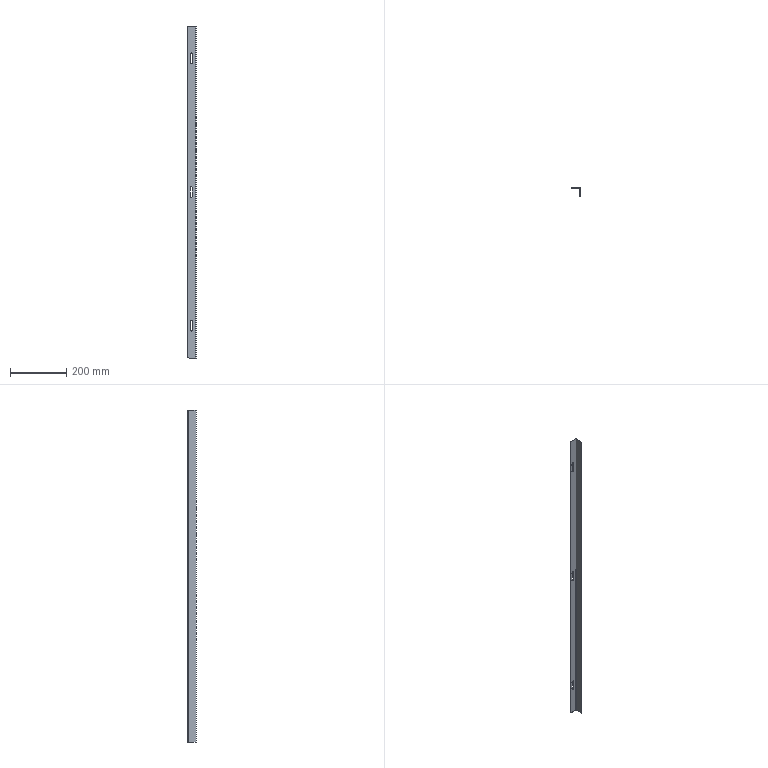Part | SolidWorks | features Cut 1, Fillet 1, FlatPattern 1, SMBaseFlange 1, SheetMetal 1 | 1 solid | 31 faces | box 30 x 30 x 1181 mm | volume 101588 mm3 | plane 18 | cylinder 13 | commonest cylinder face diameters 8 x9 10 x2 0.4 x1 3.4 x1
STEP:
#1=CARTESIAN_POINT('',(-17.5,-1.5,494.5));
#2=VERTEX_POINT('',#1);
#3=CARTESIAN_POINT('',(-13.5,-1.5,490.5));
#4=VERTEX_POINT('',#3);
#5=CARTESIAN_POINT('',(-17.5,-1.5,490.5));
#6=DIRECTION('',(0.,1.,0.));
#7=DIRECTION('',(-1.,0.,0.));
#8=AXIS2_PLACEMENT_3D('',#5,#6,#7);
#9=CIRCLE('',#8,4.);
#10=EDGE_CURVE('',#2,#4,#9,.T.);
#11=ORIENTED_EDGE('',*,*,#10,.F.);
#12=CARTESIAN_POINT('',(-17.5,0.,494.5));
#13=VERTEX_POINT('',#12);
#14=CARTESIAN_POINT('',(-17.5,-10.,494.5));
#15=DIRECTION('',(0.,1.,0.));
#16=VECTOR('',#15,1000.);
#17=LINE('',#14,#16);
#18=EDGE_CURVE('',#2,#13,#17,.T.);
#19=ORIENTED_EDGE('',*,*,#18,.T.);
#20=CARTESIAN_POINT('',(-13.5,0.,490.5));
#21=VERTEX_POINT('',#20);
#22=CARTESIAN_POINT('',(-17.5,0.,490.5));
#23=DIRECTION('',(0.,1.,0.));
#24=DIRECTION('',(0.,0.,-1.));
#25=AXIS2_PLACEMENT_3D('',#22,#23,#24);
#26=CIRCLE('',#25,4.);
#27=EDGE_CURVE('',#13,#21,#26,.T.);
#28=ORIENTED_EDGE('',*,*,#27,.T.);
#29=CARTESIAN_POINT('',(-13.5,-10.,490.5));
#30=DIRECTION('',(0.,1.,0.));
#31=VECTOR('',#30,1000.);
#32=LINE('',#29,#31);
#33=EDGE_CURVE('',#4,#21,#32,.T.);
#34=ORIENTED_EDGE('',*,*,#33,.F.);
#35=EDGE_LOOP('',(#11,#19,#28,#34));
#36=FACE_OUTER_BOUND('',#35,.T.);
#37=CARTESIAN_POINT('',(-17.5,-10.,490.5));
#38=DIRECTION('',(0.,1.,0.));
#39=DIRECTION('',(0.,0.,1.));
#40=AXIS2_PLACEMENT_3D('',#37,#38,#39);
#41=CYLINDRICAL_SURFACE('',#40,4.);
#42=ADVANCED_FACE('',(#36),#41,.F.);
#43=CARTESIAN_POINT('',(-17.5,-1.5,-456.5));
#44=VERTEX_POINT('',#43);
#45=CARTESIAN_POINT('',(-13.5,-1.5,-460.5));
#46=VERTEX_POINT('',#45);
#47=CARTESIAN_POINT('',(-17.5,-1.5,-460.5));
#48=DIRECTION('',(0.,1.,0.));
#49=DIRECTION('',(-1.,0.,0.));
#50=AXIS2_PLACEMENT_3D('',#47,#48,#49);
#51=CIRCLE('',#50,4.);
#52=EDGE_CURVE('',#44,#46,#51,.T.);
#53=ORIENTED_EDGE('',*,*,#52,.F.);
#54=CARTESIAN_POINT('',(-17.5,0.,-456.5));
#55=VERTEX_POINT('',#54);
#56=CARTESIAN_POINT('',(-17.5,-10.,-456.5));
#57=DIRECTION('',(0.,1.,0.));
#58=VECTOR('',#57,1000.);
#59=LINE('',#56,#58);
#60=EDGE_CURVE('',#44,#55,#59,.T.);
#61=ORIENTED_EDGE('',*,*,#60,.T.);
#62=CARTESIAN_POINT('',(-13.5,0.,-460.5));
#63=VERTEX_POINT('',#62);
#64=CARTESIAN_POINT('',(-17.5,0.,-460.5));
#65=DIRECTION('',(0.,1.,0.));
#66=DIRECTION('',(0.,0.,1.));
#67=AXIS2_PLACEMENT_3D('',#64,#65,#66);
#68=CIRCLE('',#67,4.);
#69=EDGE_CURVE('',#55,#63,#68,.T.);
#70=ORIENTED_EDGE('',*,*,#69,.T.);
#71=CARTESIAN_POINT('',(-13.5,-10.,-460.5));
#72=DIRECTION('',(0.,1.,0.));
#73=VECTOR('',#72,1000.);
#74=LINE('',#71,#73);
#75=EDGE_CURVE('',#46,#63,#74,.T.);
#76=ORIENTED_EDGE('',*,*,#75,.F.);
#77=EDGE_LOOP('',(#53,#61,#70,#76));
#78=FACE_OUTER_BOUND('',#77,.T.);
#79=CARTESIAN_POINT('',(-17.5,-10.,-460.5));
#80=DIRECTION('',(0.,1.,0.));
#81=DIRECTION('',(0.,0.,1.));
#82=AXIS2_PLACEMENT_3D('',#79,#80,#81);
#83=CYLINDRICAL_SURFACE('',#82,4.);
#84=ADVANCED_FACE('',(#78),#83,.F.);
#85=CARTESIAN_POINT('',(-17.5,-1.5,19.));
#86=VERTEX_POINT('',#85);
#87=CARTESIAN_POINT('',(-13.5,-1.5,15.));
#88=VERTEX_POINT('',#87);
#89=CARTESIAN_POINT('',(-17.5,-1.5,15.));
#90=DIRECTION('',(0.,1.,0.));
#91=DIRECTION('',(-1.,0.,0.));
#92=AXIS2_PLACEMENT_3D('',#89,#90,#91);
#93=CIRCLE('',#92,4.);
#94=EDGE_CURVE('',#86,#88,#93,.T.);
#95=ORIENTED_EDGE('',*,*,#94,.F.);
#96=CARTESIAN_POINT('',(-17.5,0.,19.));
#97=VERTEX_POINT('',#96);
#98=CARTESIAN_POINT('',(-17.5,-10.,19.));
#99=DIRECTION('',(0.,1.,0.));
#100=VECTOR('',#99,1000.);
#101=LINE('',#98,#100);
#102=EDGE_CURVE('',#86,#97,#101,.T.);
#103=ORIENTED_EDGE('',*,*,#102,.T.);
#104=CARTESIAN_POINT('',(-13.5,0.,15.));
#105=VERTEX_POINT('',#104);
#106=CARTESIAN_POINT('',(-17.5,0.,15.));
#107=DIRECTION('',(0.,1.,0.));
#108=DIRECTION('',(0.,0.,1.));
#109=AXIS2_PLACEMENT_3D('',#106,#107,#108);
#110=CIRCLE('',#109,4.);
#111=EDGE_CURVE('',#97,#105,#110,.T.);
#112=ORIENTED_EDGE('',*,*,#111,.T.);
#113=CARTESIAN_POINT('',(-13.5,-10.,15.));
#114=DIRECTION('',(0.,1.,0.));
#115=VECTOR('',#114,1000.);
#116=LINE('',#113,#115);
#117=EDGE_CURVE('',#88,#105,#116,.T.);
#118=ORIENTED_EDGE('',*,*,#117,.F.);
#119=EDGE_LOOP('',(#95,#103,#112,#118));
#120=FACE_OUTER_BOUND('',#119,.T.);
#121=CARTESIAN_POINT('',(-17.5,-10.,15.));
#122=DIRECTION('',(0.,1.,0.));
#123=DIRECTION('',(0.,0.,1.));
#124=AXIS2_PLACEMENT_3D('',#121,#122,#123);
#125=CYLINDRICAL_SURFACE('',#124,4.);
#126=ADVANCED_FACE('',(#120),#125,.F.);
#127=CARTESIAN_POINT('',(0.,-1.7,590.5));
#128=VERTEX_POINT('',#127);
#129=CARTESIAN_POINT('',(-1.5,-1.7,590.5));
#130=VERTEX_POINT('',#129);
#131=CARTESIAN_POINT('',(0.,-1.7,590.5));
#132=DIRECTION('',(-1.,0.,0.));
#133=VECTOR('',#132,1000.);
#134=LINE('',#131,#133);
#135=EDGE_CURVE('',#128,#130,#134,.T.);
#136=ORIENTED_EDGE('',*,*,#135,.F.);
#137=CARTESIAN_POINT('',(-1.7,0.,590.5));
#138=VERTEX_POINT('',#137);
#139=CARTESIAN_POINT('',(-1.7,-1.7,590.5));
#140=DIRECTION('',(0.,0.,-1.));
#141=DIRECTION('',(1.,0.,0.));
#142=AXIS2_PLACEMENT_3D('',#139,#140,#141);
#143=CIRCLE('',#142,1.7);
#144=EDGE_CURVE('',#138,#128,#143,.T.);
#145=ORIENTED_EDGE('',*,*,#144,.F.);
#146=CARTESIAN_POINT('',(-1.7,-1.5,590.5));
#147=VERTEX_POINT('',#146);
#148=CARTESIAN_POINT('',(-1.7,-1.5,590.5));
#149=DIRECTION('',(0.,1.,0.));
#150=VECTOR('',#149,1000.);
#151=LINE('',#148,#150);
#152=EDGE_CURVE('',#147,#138,#151,.T.);
#153=ORIENTED_EDGE('',*,*,#152,.F.);
#154=CARTESIAN_POINT('',(-1.7,-1.7,590.5));
#155=DIRECTION('',(0.,0.,-1.));
#156=DIRECTION('',(1.,0.,0.));
#157=AXIS2_PLACEMENT_3D('',#154,#155,#156);
#158=CIRCLE('',#157,0.2);
#159=EDGE_CURVE('',#147,#130,#158,.T.);
#160=ORIENTED_EDGE('',*,*,#159,.T.);
#161=EDGE_LOOP('',(#136,#145,#153,#160));
#162=FACE_OUTER_BOUND('',#161,.T.);
#163=CARTESIAN_POINT('',(0.,-1.7,590.5));
#164=DIRECTION('',(0.,0.,1.));
#165=DIRECTION('',(1.,0.,0.));
#166=AXIS2_PLACEMENT_3D('',#163,#164,#165);
#167=PLANE('',#166);
#168=ADVANCED_FACE('',(#162),#167,.T.);
#169=CARTESIAN_POINT('',(0.,-30.,590.5));
#170=VERTEX_POINT('',#169);
#171=CARTESIAN_POINT('',(0.,0.,590.5));
#172=DIRECTION('',(0.,-1.,0.));
#173=VECTOR('',#172,1000.);
#174=LINE('',#171,#173);
#175=EDGE_CURVE('',#128,#170,#174,.T.);
#176=ORIENTED_EDGE('',*,*,#175,.F.);
#177=ORIENTED_EDGE('',*,*,#135,.T.);
#178=CARTESIAN_POINT('',(-1.5,-30.,590.5));
#179=VERTEX_POINT('',#178);
#180=CARTESIAN_POINT('',(-1.5,0.,590.5));
#181=DIRECTION('',(0.,-1.,0.));
#182=VECTOR('',#181,1000.);
#183=LINE('',#180,#182);
#184=EDGE_CURVE('',#130,#179,#183,.T.);
#185=ORIENTED_EDGE('',*,*,#184,.T.);
#186=CARTESIAN_POINT('',(0.,-30.,590.5));
#187=DIRECTION('',(-1.,0.,0.));
#188=VECTOR('',#187,1000.);
#189=LINE('',#186,#188);
#190=EDGE_CURVE('',#170,#179,#189,.T.);
#191=ORIENTED_EDGE('',*,*,#190,.F.);
#192=EDGE_LOOP('',(#176,#177,#185,#191));
#193=FACE_OUTER_BOUND('',#192,.T.);
#194=CARTESIAN_POINT('',(-1.7,-1.5,590.5));
#195=DIRECTION('',(0.,0.,1.));
#196=DIRECTION('',(1.,0.,0.));
#197=AXIS2_PLACEMENT_3D('',#194,#195,#196);
#198=PLANE('',#197);
#199=ADVANCED_FACE('',(#193),#198,.T.);
#200=CARTESIAN_POINT('',(-1.7,0.,-590.5));
#201=VERTEX_POINT('',#200);
#202=CARTESIAN_POINT('',(-1.7,-1.5,-590.5));
#203=VERTEX_POINT('',#202);
#204=CARTESIAN_POINT('',(-1.7,0.,-590.5));
#205=DIRECTION('',(0.,-1.,0.));
#206=VECTOR('',#205,1000.);
#207=LINE('',#204,#206);
#208=EDGE_CURVE('',#201,#203,#207,.T.);
#209=ORIENTED_EDGE('',*,*,#208,.F.);
#210=CARTESIAN_POINT('',(0.,-1.7,-590.5));
#211=VERTEX_POINT('',#210);
#212=CARTESIAN_POINT('',(-1.7,-1.7,-590.5));
#213=DIRECTION('',(0.,0.,-1.));
#214=DIRECTION('',(1.,0.,0.));
#215=AXIS2_PLACEMENT_3D('',#212,#213,#214);
#216=CIRCLE('',#215,1.7);
#217=EDGE_CURVE('',#201,#211,#216,.T.);
#218=ORIENTED_EDGE('',*,*,#217,.T.);
#219=CARTESIAN_POINT('',(-1.5,-1.7,-590.5));
#220=VERTEX_POINT('',#219);
#221=CARTESIAN_POINT('',(-1.5,-1.7,-590.5));
#222=DIRECTION('',(1.,0.,0.));
#223=VECTOR('',#222,1000.);
#224=LINE('',#221,#223);
#225=EDGE_CURVE('',#220,#211,#224,.T.);
#226=ORIENTED_EDGE('',*,*,#225,.F.);
#227=CARTESIAN_POINT('',(-1.7,-1.7,-590.5));
#228=DIRECTION('',(0.,0.,-1.));
#229=DIRECTION('',(1.,0.,0.));
#230=AXIS2_PLACEMENT_3D('',#227,#228,#229);
#231=CIRCLE('',#230,0.2);
#232=EDGE_CURVE('',#203,#220,#231,.T.);
#233=ORIENTED_EDGE('',*,*,#232,.F.);
#234=EDGE_LOOP('',(#209,#218,#226,#233));
#235=FACE_OUTER_BOUND('',#234,.T.);
#236=CARTESIAN_POINT('',(-1.7,0.,-590.5));
#237=DIRECTION('',(0.,0.,-1.));
#238=DIRECTION('',(-1.,0.,0.));
#239=AXIS2_PLACEMENT_3D('',#236,#237,#238);
#240=PLANE('',#239);
#241=ADVANCED_FACE('',(#235),#240,.T.);
#242=CARTESIAN_POINT('',(-25.,-1.5,-590.5));
#243=VERTEX_POINT('',#242);
#244=CARTESIAN_POINT('',(0.,-1.5,-590.5));
#245=DIRECTION('',(1.,0.,0.));
#246=VECTOR('',#245,1000.);
#247=LINE('',#244,#246);
#248=EDGE_CURVE('',#243,#203,#247,.T.);
#249=ORIENTED_EDGE('',*,*,#248,.F.);
#250=CARTESIAN_POINT('',(-25.,0.,-590.5));
#251=VERTEX_POINT('',#250);
#252=CARTESIAN_POINT('',(-25.,-1.7,-590.5));
#253=DIRECTION('',(0.,1.,0.));
#254=VECTOR('',#253,1000.);
#255=LINE('',#252,#254);
#256=EDGE_CURVE('',#243,#251,#255,.T.);
#257=ORIENTED_EDGE('',*,*,#256,.T.);
#258=CARTESIAN_POINT('',(0.,0.,-590.5));
#259=DIRECTION('',(1.,0.,0.));
#260=VECTOR('',#259,1000.);
#261=LINE('',#258,#260);
#262=EDGE_CURVE('',#251,#201,#261,.T.);
#263=ORIENTED_EDGE('',*,*,#262,.T.);
#264=ORIENTED_EDGE('',*,*,#208,.T.);
#265=EDGE_LOOP('',(#249,#257,#263,#264));
#266=FACE_OUTER_BOUND('',#265,.T.);
#267=CARTESIAN_POINT('',(-1.5,-1.7,-590.5));
#268=DIRECTION('',(0.,0.,-1.));
#269=DIRECTION('',(-1.,0.,0.));
#270=AXIS2_PLACEMENT_3D('',#267,#268,#269);
#271=PLANE('',#270);
#272=ADVANCED_FACE('',(#266),#271,.T.);
#273=CARTESIAN_POINT('',(-1.5,-30.,-590.5));
#274=VERTEX_POINT('',#273);
#275=CARTESIAN_POINT('',(-1.5,0.,-590.5));
#276=DIRECTION('',(0.,-1.,0.));
#277=VECTOR('',#276,1000.);
#278=LINE('',#275,#277);
#279=EDGE_CURVE('',#220,#274,#278,.T.);
#280=ORIENTED_EDGE('',*,*,#279,.T.);
#281=CARTESIAN_POINT('',(-1.5,-30.,590.5));
#282=DIRECTION('',(0.,0.,-1.));
#283=VECTOR('',#282,1000.);
#284=LINE('',#281,#283);
#285=EDGE_CURVE('',#179,#274,#284,.T.);
#286=ORIENTED_EDGE('',*,*,#285,.F.);
#287=ORIENTED_EDGE('',*,*,#184,.F.);
#288=CARTESIAN_POINT('',(-1.5,-1.7,590.5));
#289=DIRECTION('',(0.,0.,-1.));
#290=VECTOR('',#289,1000.);
#291=LINE('',#288,#290);
#292=EDGE_CURVE('',#130,#220,#291,.T.);
#293=ORIENTED_EDGE('',*,*,#292,.T.);
#294=EDGE_LOOP('',(#280,#286,#287,#293));
#295=FACE_OUTER_BOUND('',#294,.T.);
#296=CARTESIAN_POINT('',(-1.5,0.,590.5));
#297=DIRECTION('',(1.,0.,0.));
#298=DIRECTION('',(0.,1.,0.));
#299=AXIS2_PLACEMENT_3D('',#296,#297,#298);
#300=PLANE('',#299);
#301=ADVANCED_FACE('',(#295),#300,.F.);
#302=CARTESIAN_POINT('',(0.,-30.,-590.5));
#303=VERTEX_POINT('',#302);
#304=CARTESIAN_POINT('',(0.,-30.,-590.5));
#305=DIRECTION('',(-1.,0.,0.));
#306=VECTOR('',#305,1000.);
#307=LINE('',#304,#306);
#308=EDGE_CURVE('',#303,#274,#307,.T.);
#309=ORIENTED_EDGE('',*,*,#308,.F.);
#310=CARTESIAN_POINT('',(0.,-30.,590.5));
#311=DIRECTION('',(0.,0.,-1.));
#312=VECTOR('',#311,1000.);
#313=LINE('',#310,#312);
#314=EDGE_CURVE('',#170,#303,#313,.T.);
#315=ORIENTED_EDGE('',*,*,#314,.F.);
#316=ORIENTED_EDGE('',*,*,#190,.T.);
#317=ORIENTED_EDGE('',*,*,#285,.T.);
#318=EDGE_LOOP('',(#309,#315,#316,#317));
#319=FACE_OUTER_BOUND('',#318,.T.);
#320=CARTESIAN_POINT('',(0.,-30.,590.5));
#321=DIRECTION('',(0.,-1.,0.));
#322=DIRECTION('',(0.,0.,-1.));
#323=AXIS2_PLACEMENT_3D('',#320,#321,#322);
#324=PLANE('',#323);
#325=ADVANCED_FACE('',(#319),#324,.T.);
#326=CARTESIAN_POINT('',(0.,0.,-590.5));
#327=DIRECTION('',(0.,-1.,0.));
#328=VECTOR('',#327,1000.);
#329=LINE('',#326,#328);
#330=EDGE_CURVE('',#211,#303,#329,.T.);
#331=ORIENTED_EDGE('',*,*,#330,.F.);
#332=CARTESIAN_POINT('',(0.,-1.7,590.5));
#333=DIRECTION('',(0.,0.,-1.));
#334=VECTOR('',#333,1000.);
#335=LINE('',#332,#334);
#336=EDGE_CURVE('',#128,#211,#335,.T.);
#337=ORIENTED_EDGE('',*,*,#336,.F.);
#338=ORIENTED_EDGE('',*,*,#175,.T.);
#339=ORIENTED_EDGE('',*,*,#314,.T.);
#340=EDGE_LOOP('',(#331,#337,#338,#339));
#341=FACE_OUTER_BOUND('',#340,.T.);
#342=CARTESIAN_POINT('',(0.,0.,590.5));
#343=DIRECTION('',(1.,0.,0.));
#344=DIRECTION('',(0.,1.,0.));
#345=AXIS2_PLACEMENT_3D('',#342,#343,#344);
#346=PLANE('',#345);
#347=ADVANCED_FACE('',(#341),#346,.T.);
#348=ORIENTED_EDGE('',*,*,#217,.F.);
#349=CARTESIAN_POINT('',(-1.7,0.,590.5));
#350=DIRECTION('',(0.,0.,-1.));
#351=VECTOR('',#350,1000.);
#352=LINE('',#349,#351);
#353=EDGE_CURVE('',#138,#201,#352,.T.);
#354=ORIENTED_EDGE('',*,*,#353,.F.);
#355=ORIENTED_EDGE('',*,*,#144,.T.);
#356=ORIENTED_EDGE('',*,*,#336,.T.);
#357=EDGE_LOOP('',(#348,#354,#355,#356));
#358=FACE_OUTER_BOUND('',#357,.T.);
#359=CARTESIAN_POINT('',(-1.7,-1.7,590.5));
#360=DIRECTION('',(0.,0.,-1.));
#361=DIRECTION('',(-1.,0.,0.));
#362=AXIS2_PLACEMENT_3D('',#359,#360,#361);
#363=CYLINDRICAL_SURFACE('',#362,1.7);
#364=ADVANCED_FACE('',(#358),#363,.T.);
#365=CARTESIAN_POINT('',(-13.5,0.,460.5));
#366=VERTEX_POINT('',#365);
#367=CARTESIAN_POINT('',(-21.5,0.,460.5));
#368=VERTEX_POINT('',#367);
#369=CARTESIAN_POINT('',(-17.5,0.,460.5));
#370=DIRECTION('',(0.,1.,0.));
#371=DIRECTION('',(0.,0.,-1.));
#372=AXIS2_PLACEMENT_3D('',#369,#370,#371);
#373=CIRCLE('',#372,4.);
#374=EDGE_CURVE('',#366,#368,#373,.T.);
#375=ORIENTED_EDGE('',*,*,#374,.F.);
#376=CARTESIAN_POINT('',(-13.5,0.,460.5));
#377=DIRECTION('',(0.,0.,-1.));
#378=VECTOR('',#377,1000.);
#379=LINE('',#376,#378);
#380=EDGE_CURVE('',#21,#366,#379,.T.);
#381=ORIENTED_EDGE('',*,*,#380,.F.);
#382=ORIENTED_EDGE('',*,*,#27,.F.);
#383=CARTESIAN_POINT('',(-21.5,0.,490.5));
#384=VERTEX_POINT('',#383);
#385=CARTESIAN_POINT('',(-17.5,0.,490.5));
#386=DIRECTION('',(0.,1.,0.));
#387=DIRECTION('',(0.,0.,-1.));
#388=AXIS2_PLACEMENT_3D('',#385,#386,#387);
#389=CIRCLE('',#388,4.);
#390=EDGE_CURVE('',#384,#13,#389,.T.);
#391=ORIENTED_EDGE('',*,*,#390,.F.);
#392=CARTESIAN_POINT('',(-21.5,0.,460.5));
#393=DIRECTION('',(0.,0.,1.));
#394=VECTOR('',#393,1000.);
#395=LINE('',#392,#394);
#396=EDGE_CURVE('',#368,#384,#395,.T.);
#397=ORIENTED_EDGE('',*,*,#396,.F.);
#398=EDGE_LOOP('',(#375,#381,#382,#391,#397));
#399=FACE_BOUND('',#398,.T.);
#400=CARTESIAN_POINT('',(-21.5,0.,-460.5));
#401=VERTEX_POINT('',#400);
#402=CARTESIAN_POINT('',(-17.5,0.,-460.5));
#403=DIRECTION('',(0.,1.,0.));
#404=DIRECTION('',(0.,0.,1.));
#405=AXIS2_PLACEMENT_3D('',#402,#403,#404);
#406=CIRCLE('',#405,4.);
#407=EDGE_CURVE('',#401,#55,#406,.T.);
#408=ORIENTED_EDGE('',*,*,#407,.F.);
#409=CARTESIAN_POINT('',(-21.5,0.,-490.5));
#410=VERTEX_POINT('',#409);
#411=CARTESIAN_POINT('',(-21.5,0.,-460.5));
#412=DIRECTION('',(0.,0.,1.));
#413=VECTOR('',#412,1000.);
#414=LINE('',#411,#413);
#415=EDGE_CURVE('',#410,#401,#414,.T.);
#416=ORIENTED_EDGE('',*,*,#415,.F.);
#417=CARTESIAN_POINT('',(-13.5,0.,-490.5));
#418=VERTEX_POINT('',#417);
#419=CARTESIAN_POINT('',(-17.5,0.,-490.5));
#420=DIRECTION('',(0.,1.,0.));
#421=DIRECTION('',(0.,0.,1.));
#422=AXIS2_PLACEMENT_3D('',#419,#420,#421);
#423=CIRCLE('',#422,4.);
#424=EDGE_CURVE('',#418,#410,#423,.T.);
#425=ORIENTED_EDGE('',*,*,#424,.F.);
#426=CARTESIAN_POINT('',(-13.5,0.,-460.5));
#427=DIRECTION('',(0.,0.,-1.));
#428=VECTOR('',#427,1000.);
#429=LINE('',#426,#428);
#430=EDGE_CURVE('',#63,#418,#429,.T.);
#431=ORIENTED_EDGE('',*,*,#430,.F.);
#432=ORIENTED_EDGE('',*,*,#69,.F.);
#433=EDGE_LOOP('',(#408,#416,#425,#431,#432));
#434=FACE_BOUND('',#433,.T.);
#435=CARTESIAN_POINT('',(-21.5,0.,15.));
#436=VERTEX_POINT('',#435);
#437=CARTESIAN_POINT('',(-17.5,0.,15.));
#438=DIRECTION('',(0.,1.,0.));
#439=DIRECTION('',(0.,0.,1.));
#440=AXIS2_PLACEMENT_3D('',#437,#438,#439);
#441=CIRCLE('',#440,4.);
#442=EDGE_CURVE('',#436,#97,#441,.T.);
#443=ORIENTED_EDGE('',*,*,#442,.F.);
#444=CARTESIAN_POINT('',(-21.5,0.,-15.));
#445=VERTEX_POINT('',#444);
#446=CARTESIAN_POINT('',(-21.5,0.,15.));
#447=DIRECTION('',(0.,0.,1.));
#448=VECTOR('',#447,1000.);
#449=LINE('',#446,#448);
#450=EDGE_CURVE('',#445,#436,#449,.T.);
#451=ORIENTED_EDGE('',*,*,#450,.F.);
#452=CARTESIAN_POINT('',(-13.5,0.,-15.));
#453=VERTEX_POINT('',#452);
#454=CARTESIAN_POINT('',(-17.5,0.,-15.));
#455=DIRECTION('',(0.,1.,0.));
#456=DIRECTION('',(0.,0.,1.));
#457=AXIS2_PLACEMENT_3D('',#454,#455,#456);
#458=CIRCLE('',#457,4.);
#459=EDGE_CURVE('',#453,#445,#458,.T.);
#460=ORIENTED_EDGE('',*,*,#459,.F.);
#461=CARTESIAN_POINT('',(-13.5,0.,15.));
#462=DIRECTION('',(0.,0.,-1.));
#463=VECTOR('',#462,1000.);
#464=LINE('',#461,#463);
#465=EDGE_CURVE('',#105,#453,#464,.T.);
#466=ORIENTED_EDGE('',*,*,#465,.F.);
#467=ORIENTED_EDGE('',*,*,#111,.F.);
#468=EDGE_LOOP('',(#443,#451,#460,#466,#467));
#469=FACE_BOUND('',#468,.T.);
#470=ORIENTED_EDGE('',*,*,#262,.F.);
#471=CARTESIAN_POINT('',(-30.,0.,-585.5));
#472=VERTEX_POINT('',#471);
#473=CARTESIAN_POINT('',(-25.,0.,-585.5));
#474=DIRECTION('',(0.,1.,0.));
#475=DIRECTION('',(-1.,0.,0.));
#476=AXIS2_PLACEMENT_3D('',#473,#474,#475);
#477=CIRCLE('',#476,5.);
#478=EDGE_CURVE('',#251,#472,#477,.T.);
#479=ORIENTED_EDGE('',*,*,#478,.T.);
#480=CARTESIAN_POINT('',(-30.,0.,585.5));
#481=VERTEX_POINT('',#480);
#482=CARTESIAN_POINT('',(-30.,0.,590.5));
#483=DIRECTION('',(0.,0.,-1.));
#484=VECTOR('',#483,1000.);
#485=LINE('',#482,#484);
#486=EDGE_CURVE('',#481,#472,#485,.T.);
#487=ORIENTED_EDGE('',*,*,#486,.F.);
#488=CARTESIAN_POINT('',(-25.,0.,590.5));
#489=VERTEX_POINT('',#488);
#490=CARTESIAN_POINT('',(-25.,0.,585.5));
#491=DIRECTION('',(0.,1.,0.));
#492=DIRECTION('',(-1.,0.,0.));
#493=AXIS2_PLACEMENT_3D('',#490,#491,#492);
#494=CIRCLE('',#493,5.);
#495=EDGE_CURVE('',#481,#489,#494,.T.);
#496=ORIENTED_EDGE('',*,*,#495,.T.);
#497=CARTESIAN_POINT('',(0.,0.,590.5));
#498=DIRECTION('',(1.,0.,0.));
#499=VECTOR('',#498,1000.);
#500=LINE('',#497,#499);
#501=EDGE_CURVE('',#489,#138,#500,.T.);
#502=ORIENTED_EDGE('',*,*,#501,.T.);
#503=ORIENTED_EDGE('',*,*,#353,.T.);
#504=EDGE_LOOP('',(#470,#479,#487,#496,#502,#503));
#505=FACE_OUTER_BOUND('',#504,.T.);
#506=CARTESIAN_POINT('',(0.,0.,590.5));
#507=DIRECTION('',(0.,1.,0.));
#508=DIRECTION('',(-1.,0.,0.));
#509=AXIS2_PLACEMENT_3D('',#506,#507,#508);
#510=PLANE('',#509);
#511=ADVANCED_FACE('',(#399,#434,#469,#505),#510,.T.);
#512=ORIENTED_EDGE('',*,*,#486,.T.);
#513=CARTESIAN_POINT('',(-30.,-1.5,-585.5));
#514=VERTEX_POINT('',#513);
#515=CARTESIAN_POINT('',(-30.,-1.5,-585.5));
#516=DIRECTION('',(0.,-1.,0.));
#517=VECTOR('',#516,1000.);
#518=LINE('',#515,#517);
#519=EDGE_CURVE('',#472,#514,#518,.T.);
#520=ORIENTED_EDGE('',*,*,#519,.T.);
#521=CARTESIAN_POINT('',(-30.,-1.5,585.5));
#522=VERTEX_POINT('',#521);
#523=CARTESIAN_POINT('',(-30.,-1.5,590.5));
#524=DIRECTION('',(0.,0.,-1.));
#525=VECTOR('',#524,1000.);
#526=LINE('',#523,#525);
#527=EDGE_CURVE('',#522,#514,#526,.T.);
#528=ORIENTED_EDGE('',*,*,#527,.F.);
#529=CARTESIAN_POINT('',(-30.,-1.5,585.5));
#530=DIRECTION('',(0.,1.,0.));
#531=VECTOR('',#530,1000.);
#532=LINE('',#529,#531);
#533=EDGE_CURVE('',#522,#481,#532,.T.);
#534=ORIENTED_EDGE('',*,*,#533,.T.);
#535=EDGE_LOOP('',(#512,#520,#528,#534));
#536=FACE_OUTER_BOUND('',#535,.T.);
#537=CARTESIAN_POINT('',(-30.,-1.5,590.5));
#538=DIRECTION('',(-1.,0.,0.));
#539=DIRECTION('',(0.,0.,1.));
#540=AXIS2_PLACEMENT_3D('',#537,#538,#539);
#541=PLANE('',#540);
#542=ADVANCED_FACE('',(#536),#541,.T.);
#543=CARTESIAN_POINT('',(-13.5,-1.5,460.5));
#544=VERTEX_POINT('',#543);
#545=CARTESIAN_POINT('',(-13.5,-1.5,590.5));
#546=DIRECTION('',(0.,0.,-1.));
#547=VECTOR('',#546,1000.);
#548=LINE('',#545,#547);
#549=EDGE_CURVE('',#4,#544,#548,.T.);
#550=ORIENTED_EDGE('',*,*,#549,.T.);
#551=CARTESIAN_POINT('',(-21.5,-1.5,460.5));
#552=VERTEX_POINT('',#551);
#553=CARTESIAN_POINT('',(-17.5,-1.5,460.5));
#554=DIRECTION('',(0.,1.,0.));
#555=DIRECTION('',(-1.,0.,0.));
#556=AXIS2_PLACEMENT_3D('',#553,#554,#555);
#557=CIRCLE('',#556,4.);
#558=EDGE_CURVE('',#544,#552,#557,.T.);
#559=ORIENTED_EDGE('',*,*,#558,.T.);
#560=CARTESIAN_POINT('',(-21.5,-1.5,490.5));
#561=VERTEX_POINT('',#560);
#562=CARTESIAN_POINT('',(-21.5,-1.5,590.5));
#563=DIRECTION('',(0.,0.,1.));
#564=VECTOR('',#563,1000.);
#565=LINE('',#562,#564);
#566=EDGE_CURVE('',#552,#561,#565,.T.);
#567=ORIENTED_EDGE('',*,*,#566,.T.);
#568=CARTESIAN_POINT('',(-17.5,-1.5,490.5));
#569=DIRECTION('',(0.,1.,0.));
#570=DIRECTION('',(-1.,0.,0.));
#571=AXIS2_PLACEMENT_3D('',#568,#569,#570);
#572=CIRCLE('',#571,4.);
#573=EDGE_CURVE('',#561,#2,#572,.T.);
#574=ORIENTED_EDGE('',*,*,#573,.T.);
#575=ORIENTED_EDGE('',*,*,#10,.T.);
#576=EDGE_LOOP('',(#550,#559,#567,#574,#575));
#577=FACE_BOUND('',#576,.T.);
#578=CARTESIAN_POINT('',(-21.5,-1.5,-490.5));
#579=VERTEX_POINT('',#578);
#580=CARTESIAN_POINT('',(-21.5,-1.5,-460.5));
#581=VERTEX_POINT('',#580);
#582=CARTESIAN_POINT('',(-21.5,-1.5,590.5));
#583=DIRECTION('',(0.,0.,1.));
#584=VECTOR('',#583,1000.);
#585=LINE('',#582,#584);
#586=EDGE_CURVE('',#579,#581,#585,.T.);
#587=ORIENTED_EDGE('',*,*,#586,.T.);
#588=CARTESIAN_POINT('',(-17.5,-1.5,-460.5));
#589=DIRECTION('',(0.,1.,0.));
#590=DIRECTION('',(-1.,0.,0.));
#591=AXIS2_PLACEMENT_3D('',#588,#589,#590);
#592=CIRCLE('',#591,4.);
#593=EDGE_CURVE('',#581,#44,#592,.T.);
#594=ORIENTED_EDGE('',*,*,#593,.T.);
#595=ORIENTED_EDGE('',*,*,#52,.T.);
#596=CARTESIAN_POINT('',(-13.5,-1.5,-490.5));
#597=VERTEX_POINT('',#596);
#598=CARTESIAN_POINT('',(-13.5,-1.5,590.5));
#599=DIRECTION('',(0.,0.,-1.));
#600=VECTOR('',#599,1000.);
#601=LINE('',#598,#600);
#602=EDGE_CURVE('',#46,#597,#601,.T.);
#603=ORIENTED_EDGE('',*,*,#602,.T.);
#604=CARTESIAN_POINT('',(-17.5,-1.5,-490.5));
#605=DIRECTION('',(0.,1.,0.));
#606=DIRECTION('',(-1.,0.,0.));
#607=AXIS2_PLACEMENT_3D('',#604,#605,#606);
#608=CIRCLE('',#607,4.);
#609=EDGE_CURVE('',#597,#579,#608,.T.);
#610=ORIENTED_EDGE('',*,*,#609,.T.);
#611=EDGE_LOOP('',(#587,#594,#595,#603,#610));
#612=FACE_BOUND('',#611,.T.);
#613=CARTESIAN_POINT('',(-21.5,-1.5,-15.));
#614=VERTEX_POINT('',#613);
#615=CARTESIAN_POINT('',(-21.5,-1.5,15.));
#616=VERTEX_POINT('',#615);
#617=CARTESIAN_POINT('',(-21.5,-1.5,590.5));
#618=DIRECTION('',(0.,0.,1.));
#619=VECTOR('',#618,1000.);
#620=LINE('',#617,#619);
#621=EDGE_CURVE('',#614,#616,#620,.T.);
#622=ORIENTED_EDGE('',*,*,#621,.T.);
#623=CARTESIAN_POINT('',(-17.5,-1.5,15.));
#624=DIRECTION('',(0.,1.,0.));
#625=DIRECTION('',(-1.,0.,0.));
#626=AXIS2_PLACEMENT_3D('',#623,#624,#625);
#627=CIRCLE('',#626,4.);
#628=EDGE_CURVE('',#616,#86,#627,.T.);
#629=ORIENTED_EDGE('',*,*,#628,.T.);
#630=ORIENTED_EDGE('',*,*,#94,.T.);
#631=CARTESIAN_POINT('',(-13.5,-1.5,-15.));
#632=VERTEX_POINT('',#631);
#633=CARTESIAN_POINT('',(-13.5,-1.5,590.5));
#634=DIRECTION('',(0.,0.,-1.));
#635=VECTOR('',#634,1000.);
#636=LINE('',#633,#635);
#637=EDGE_CURVE('',#88,#632,#636,.T.);
#638=ORIENTED_EDGE('',*,*,#637,.T.);
#639=CARTESIAN_POINT('',(-17.5,-1.5,-15.));
#640=DIRECTION('',(0.,1.,0.));
#641=DIRECTION('',(-1.,0.,0.));
#642=AXIS2_PLACEMENT_3D('',#639,#640,#641);
#643=CIRCLE('',#642,4.);
#644=EDGE_CURVE('',#632,#614,#643,.T.);
#645=ORIENTED_EDGE('',*,*,#644,.T.);
#646=EDGE_LOOP('',(#622,#629,#630,#638,#645));
#647=FACE_BOUND('',#646,.T.);
#648=ORIENTED_EDGE('',*,*,#527,.T.);
#649=CARTESIAN_POINT('',(-25.,-1.5,-585.5));
#650=DIRECTION('',(0.,-1.,0.));
#651=DIRECTION('',(-1.,0.,0.));
#652=AXIS2_PLACEMENT_3D('',#649,#650,#651);
#653=CIRCLE('',#652,5.);
#654=EDGE_CURVE('',#514,#243,#653,.T.);
#655=ORIENTED_EDGE('',*,*,#654,.T.);
#656=ORIENTED_EDGE('',*,*,#248,.T.);
#657=CARTESIAN_POINT('',(-1.7,-1.5,590.5));
#658=DIRECTION('',(0.,0.,-1.));
#659=VECTOR('',#658,1000.);
#660=LINE('',#657,#659);
#661=EDGE_CURVE('',#147,#203,#660,.T.);
#662=ORIENTED_EDGE('',*,*,#661,.F.);
#663=CARTESIAN_POINT('',(-25.,-1.5,590.5));
#664=VERTEX_POINT('',#663);
#665=CARTESIAN_POINT('',(0.,-1.5,590.5));
#666=DIRECTION('',(1.,0.,0.));
#667=VECTOR('',#666,1000.);
#668=LINE('',#665,#667);
#669=EDGE_CURVE('',#664,#147,#668,.T.);
#670=ORIENTED_EDGE('',*,*,#669,.F.);
#671=CARTESIAN_POINT('',(-25.,-1.5,585.5));
#672=DIRECTION('',(0.,-1.,0.));
#673=DIRECTION('',(-1.,0.,0.));
#674=AXIS2_PLACEMENT_3D('',#671,#672,#673);
#675=CIRCLE('',#674,5.);
#676=EDGE_CURVE('',#664,#522,#675,.T.);
#677=ORIENTED_EDGE('',*,*,#676,.T.);
#678=EDGE_LOOP('',(#648,#655,#656,#662,#670,#677));
#679=FACE_OUTER_BOUND('',#678,.T.);
#680=CARTESIAN_POINT('',(0.,-1.5,590.5));
#681=DIRECTION('',(0.,1.,0.));
#682=DIRECTION('',(-1.,0.,0.));
#683=AXIS2_PLACEMENT_3D('',#680,#681,#682);
#684=PLANE('',#683);
#685=ADVANCED_FACE('',(#577,#612,#647,#679),#684,.F.);
#686=ORIENTED_EDGE('',*,*,#232,.T.);
#687=ORIENTED_EDGE('',*,*,#292,.F.);
#688=ORIENTED_EDGE('',*,*,#159,.F.);
#689=ORIENTED_EDGE('',*,*,#661,.T.);
#690=EDGE_LOOP('',(#686,#687,#688,#689));
#691=FACE_OUTER_BOUND('',#690,.T.);
#692=CARTESIAN_POINT('',(-1.7,-1.7,590.5));
#693=DIRECTION('',(0.,0.,-1.));
#694=DIRECTION('',(-1.,0.,0.));
#695=AXIS2_PLACEMENT_3D('',#692,#693,#694);
#696=CYLINDRICAL_SURFACE('',#695,0.2);
#697=ADVANCED_FACE('',(#691),#696,.F.);
#698=ORIENTED_EDGE('',*,*,#501,.F.);
#699=CARTESIAN_POINT('',(-25.,-1.7,590.5));
#700=DIRECTION('',(0.,-1.,0.));
#701=VECTOR('',#700,1000.);
#702=LINE('',#699,#701);
#703=EDGE_CURVE('',#489,#664,#702,.T.);
#704=ORIENTED_EDGE('',*,*,#703,.T.);
#705=ORIENTED_EDGE('',*,*,#669,.T.);
#706=ORIENTED_EDGE('',*,*,#152,.T.);
#707=EDGE_LOOP('',(#698,#704,#705,#706));
#708=FACE_OUTER_BOUND('',#707,.T.);
#709=CARTESIAN_POINT('',(-1.7,-1.7,590.5));
#710=DIRECTION('',(0.,0.,1.));
#711=DIRECTION('',(1.,0.,0.));
#712=AXIS2_PLACEMENT_3D('',#709,#710,#711);
#713=PLANE('',#712);
#714=ADVANCED_FACE('',(#708),#713,.T.);
#715=ORIENTED_EDGE('',*,*,#279,.F.);
#716=ORIENTED_EDGE('',*,*,#225,.T.);
#717=ORIENTED_EDGE('',*,*,#330,.T.);
#718=ORIENTED_EDGE('',*,*,#308,.T.);
#719=EDGE_LOOP('',(#715,#716,#717,#718));
#720=FACE_OUTER_BOUND('',#719,.T.);
#721=CARTESIAN_POINT('',(-1.7,-1.7,-590.5));
#722=DIRECTION('',(0.,0.,1.));
#723=DIRECTION('',(1.,0.,0.));
#724=AXIS2_PLACEMENT_3D('',#721,#722,#723);
#725=PLANE('',#724);
#726=ADVANCED_FACE('',(#720),#725,.F.);
#727=ORIENTED_EDGE('',*,*,#102,.F.);
#728=ORIENTED_EDGE('',*,*,#628,.F.);
#729=CARTESIAN_POINT('',(-21.5,-10.,15.));
#730=DIRECTION('',(0.,1.,0.));
#731=VECTOR('',#730,1000.);
#732=LINE('',#729,#731);
#733=EDGE_CURVE('',#616,#436,#732,.T.);
#734=ORIENTED_EDGE('',*,*,#733,.T.);
#735=ORIENTED_EDGE('',*,*,#442,.T.);
#736=EDGE_LOOP('',(#727,#728,#734,#735));
#737=FACE_OUTER_BOUND('',#736,.T.);
#738=CARTESIAN_POINT('',(-17.5,-10.,15.));
#739=DIRECTION('',(0.,1.,0.));
#740=DIRECTION('',(0.,0.,1.));
#741=AXIS2_PLACEMENT_3D('',#738,#739,#740);
#742=CYLINDRICAL_SURFACE('',#741,4.);
#743=ADVANCED_FACE('',(#737),#742,.F.);
#744=CARTESIAN_POINT('',(-21.5,-10.,-15.));
#745=DIRECTION('',(0.,1.,0.));
#746=VECTOR('',#745,1000.);
#747=LINE('',#744,#746);
#748=EDGE_CURVE('',#614,#445,#747,.T.);
#749=ORIENTED_EDGE('',*,*,#748,.T.);
#750=ORIENTED_EDGE('',*,*,#450,.T.);
#751=ORIENTED_EDGE('',*,*,#733,.F.);
#752=ORIENTED_EDGE('',*,*,#621,.F.);
#753=EDGE_LOOP('',(#749,#750,#751,#752));
#754=FACE_OUTER_BOUND('',#753,.T.);
#755=CARTESIAN_POINT('',(-21.5,-10.,15.));
#756=DIRECTION('',(-1.,0.,0.));
#757=DIRECTION('',(0.,0.,1.));
#758=AXIS2_PLACEMENT_3D('',#755,#756,#757);
#759=PLANE('',#758);
#760=ADVANCED_FACE('',(#754),#759,.F.);
#761=CARTESIAN_POINT('',(-13.5,-10.,-15.));
#762=DIRECTION('',(0.,1.,0.));
#763=VECTOR('',#762,1000.);
#764=LINE('',#761,#763);
#765=EDGE_CURVE('',#632,#453,#764,.T.);
#766=ORIENTED_EDGE('',*,*,#765,.T.);
#767=ORIENTED_EDGE('',*,*,#459,.T.);
#768=ORIENTED_EDGE('',*,*,#748,.F.);
#769=ORIENTED_EDGE('',*,*,#644,.F.);
#770=EDGE_LOOP('',(#766,#767,#768,#769));
#771=FACE_OUTER_BOUND('',#770,.T.);
#772=CARTESIAN_POINT('',(-17.5,-10.,-15.));
#773=DIRECTION('',(0.,1.,0.));
#774=DIRECTION('',(0.,0.,1.));
#775=AXIS2_PLACEMENT_3D('',#772,#773,#774);
#776=CYLINDRICAL_SURFACE('',#775,4.);
#777=ADVANCED_FACE('',(#771),#776,.F.);
#778=ORIENTED_EDGE('',*,*,#117,.T.);
#779=ORIENTED_EDGE('',*,*,#465,.T.);
#780=ORIENTED_EDGE('',*,*,#765,.F.);
#781=ORIENTED_EDGE('',*,*,#637,.F.);
#782=EDGE_LOOP('',(#778,#779,#780,#781));
#783=FACE_OUTER_BOUND('',#782,.T.);
#784=CARTESIAN_POINT('',(-13.5,-10.,15.));
#785=DIRECTION('',(1.,0.,0.));
#786=DIRECTION('',(0.,0.,-1.));
#787=AXIS2_PLACEMENT_3D('',#784,#785,#786);
#788=PLANE('',#787);
#789=ADVANCED_FACE('',(#783),#788,.F.);
#790=ORIENTED_EDGE('',*,*,#60,.F.);
#791=ORIENTED_EDGE('',*,*,#593,.F.);
#792=CARTESIAN_POINT('',(-21.5,-10.,-460.5));
#793=DIRECTION('',(0.,1.,0.));
#794=VECTOR('',#793,1000.);
#795=LINE('',#792,#794);
#796=EDGE_CURVE('',#581,#401,#795,.T.);
#797=ORIENTED_EDGE('',*,*,#796,.T.);
#798=ORIENTED_EDGE('',*,*,#407,.T.);
#799=EDGE_LOOP('',(#790,#791,#797,#798));
#800=FACE_OUTER_BOUND('',#799,.T.);
#801=CARTESIAN_POINT('',(-17.5,-10.,-460.5));
#802=DIRECTION('',(0.,1.,0.));
#803=DIRECTION('',(0.,0.,1.));
#804=AXIS2_PLACEMENT_3D('',#801,#802,#803);
#805=CYLINDRICAL_SURFACE('',#804,4.);
#806=ADVANCED_FACE('',(#800),#805,.F.);
#807=CARTESIAN_POINT('',(-21.5,-10.,-490.5));
#808=DIRECTION('',(0.,1.,0.));
#809=VECTOR('',#808,1000.);
#810=LINE('',#807,#809);
#811=EDGE_CURVE('',#579,#410,#810,.T.);
#812=ORIENTED_EDGE('',*,*,#811,.T.);
#813=ORIENTED_EDGE('',*,*,#415,.T.);
#814=ORIENTED_EDGE('',*,*,#796,.F.);
#815=ORIENTED_EDGE('',*,*,#586,.F.);
#816=EDGE_LOOP('',(#812,#813,#814,#815));
#817=FACE_OUTER_BOUND('',#816,.T.);
#818=CARTESIAN_POINT('',(-21.5,-10.,-460.5));
#819=DIRECTION('',(-1.,0.,0.));
#820=DIRECTION('',(0.,0.,1.));
#821=AXIS2_PLACEMENT_3D('',#818,#819,#820);
#822=PLANE('',#821);
#823=ADVANCED_FACE('',(#817),#822,.F.);
#824=CARTESIAN_POINT('',(-13.5,-10.,-490.5));
#825=DIRECTION('',(0.,1.,0.));
#826=VECTOR('',#825,1000.);
#827=LINE('',#824,#826);
#828=EDGE_CURVE('',#597,#418,#827,.T.);
#829=ORIENTED_EDGE('',*,*,#828,.T.);
#830=ORIENTED_EDGE('',*,*,#424,.T.);
#831=ORIENTED_EDGE('',*,*,#811,.F.);
#832=ORIENTED_EDGE('',*,*,#609,.F.);
#833=EDGE_LOOP('',(#829,#830,#831,#832));
#834=FACE_OUTER_BOUND('',#833,.T.);
#835=CARTESIAN_POINT('',(-17.5,-10.,-490.5));
#836=DIRECTION('',(0.,1.,0.));
#837=DIRECTION('',(0.,0.,1.));
#838=AXIS2_PLACEMENT_3D('',#835,#836,#837);
#839=CYLINDRICAL_SURFACE('',#838,4.);
#840=ADVANCED_FACE('',(#834),#839,.F.);
#841=ORIENTED_EDGE('',*,*,#75,.T.);
#842=ORIENTED_EDGE('',*,*,#430,.T.);
#843=ORIENTED_EDGE('',*,*,#828,.F.);
#844=ORIENTED_EDGE('',*,*,#602,.F.);
#845=EDGE_LOOP('',(#841,#842,#843,#844));
#846=FACE_OUTER_BOUND('',#845,.T.);
#847=CARTESIAN_POINT('',(-13.5,-10.,-460.5));
#848=DIRECTION('',(1.,0.,0.));
#849=DIRECTION('',(0.,0.,-1.));
#850=AXIS2_PLACEMENT_3D('',#847,#848,#849);
#851=PLANE('',#850);
#852=ADVANCED_FACE('',(#846),#851,.F.);
#853=CARTESIAN_POINT('',(-13.5,-10.,460.5));
#854=DIRECTION('',(0.,1.,0.));
#855=VECTOR('',#854,1000.);
#856=LINE('',#853,#855);
#857=EDGE_CURVE('',#544,#366,#856,.T.);
#858=ORIENTED_EDGE('',*,*,#857,.T.);
#859=ORIENTED_EDGE('',*,*,#374,.T.);
#860=CARTESIAN_POINT('',(-21.5,-10.,460.5));
#861=DIRECTION('',(0.,1.,0.));
#862=VECTOR('',#861,1000.);
#863=LINE('',#860,#862);
#864=EDGE_CURVE('',#552,#368,#863,.T.);
#865=ORIENTED_EDGE('',*,*,#864,.F.);
#866=ORIENTED_EDGE('',*,*,#558,.F.);
#867=EDGE_LOOP('',(#858,#859,#865,#866));
#868=FACE_OUTER_BOUND('',#867,.T.);
#869=CARTESIAN_POINT('',(-17.5,-10.,460.5));
#870=DIRECTION('',(0.,1.,0.));
#871=DIRECTION('',(0.,0.,1.));
#872=AXIS2_PLACEMENT_3D('',#869,#870,#871);
#873=CYLINDRICAL_SURFACE('',#872,4.);
#874=ADVANCED_FACE('',(#868),#873,.F.);
#875=ORIENTED_EDGE('',*,*,#33,.T.);
#876=ORIENTED_EDGE('',*,*,#380,.T.);
#877=ORIENTED_EDGE('',*,*,#857,.F.);
#878=ORIENTED_EDGE('',*,*,#549,.F.);
#879=EDGE_LOOP('',(#875,#876,#877,#878));
#880=FACE_OUTER_BOUND('',#879,.T.);
#881=CARTESIAN_POINT('',(-13.5,-10.,460.5));
#882=DIRECTION('',(1.,0.,0.));
#883=DIRECTION('',(0.,0.,-1.));
#884=AXIS2_PLACEMENT_3D('',#881,#882,#883);
#885=PLANE('',#884);
#886=ADVANCED_FACE('',(#880),#885,.F.);
#887=ORIENTED_EDGE('',*,*,#18,.F.);
#888=ORIENTED_EDGE('',*,*,#573,.F.);
#889=CARTESIAN_POINT('',(-21.5,-10.,490.5));
#890=DIRECTION('',(0.,1.,0.));
#891=VECTOR('',#890,1000.);
#892=LINE('',#889,#891);
#893=EDGE_CURVE('',#561,#384,#892,.T.);
#894=ORIENTED_EDGE('',*,*,#893,.T.);
#895=ORIENTED_EDGE('',*,*,#390,.T.);
#896=EDGE_LOOP('',(#887,#888,#894,#895));
#897=FACE_OUTER_BOUND('',#896,.T.);
#898=CARTESIAN_POINT('',(-17.5,-10.,490.5));
#899=DIRECTION('',(0.,1.,0.));
#900=DIRECTION('',(0.,0.,1.));
#901=AXIS2_PLACEMENT_3D('',#898,#899,#900);
#902=CYLINDRICAL_SURFACE('',#901,4.);
#903=ADVANCED_FACE('',(#897),#902,.F.);
#904=ORIENTED_EDGE('',*,*,#864,.T.);
#905=ORIENTED_EDGE('',*,*,#396,.T.);
#906=ORIENTED_EDGE('',*,*,#893,.F.);
#907=ORIENTED_EDGE('',*,*,#566,.F.);
#908=EDGE_LOOP('',(#904,#905,#906,#907));
#909=FACE_OUTER_BOUND('',#908,.T.);
#910=CARTESIAN_POINT('',(-21.5,-10.,460.5));
#911=DIRECTION('',(-1.,0.,0.));
#912=DIRECTION('',(0.,0.,1.));
#913=AXIS2_PLACEMENT_3D('',#910,#911,#912);
#914=PLANE('',#913);
#915=ADVANCED_FACE('',(#909),#914,.F.);
#916=ORIENTED_EDGE('',*,*,#654,.F.);
#917=ORIENTED_EDGE('',*,*,#519,.F.);
#918=ORIENTED_EDGE('',*,*,#478,.F.);
#919=ORIENTED_EDGE('',*,*,#256,.F.);
#920=EDGE_LOOP('',(#916,#917,#918,#919));
#921=FACE_OUTER_BOUND('',#920,.T.);
#922=CARTESIAN_POINT('',(-25.,-1.7,-585.5));
#923=DIRECTION('',(0.,1.,0.));
#924=DIRECTION('',(0.,0.,1.));
#925=AXIS2_PLACEMENT_3D('',#922,#923,#924);
#926=CYLINDRICAL_SURFACE('',#925,5.);
#927=ADVANCED_FACE('',(#921),#926,.T.);
#928=ORIENTED_EDGE('',*,*,#676,.F.);
#929=ORIENTED_EDGE('',*,*,#703,.F.);
#930=ORIENTED_EDGE('',*,*,#495,.F.);
#931=ORIENTED_EDGE('',*,*,#533,.F.);
#932=EDGE_LOOP('',(#928,#929,#930,#931));
#933=FACE_OUTER_BOUND('',#932,.T.);
#934=CARTESIAN_POINT('',(-25.,-1.5,585.5));
#935=DIRECTION('',(0.,1.,0.));
#936=DIRECTION('',(0.,0.,1.));
#937=AXIS2_PLACEMENT_3D('',#934,#935,#936);
#938=CYLINDRICAL_SURFACE('',#937,5.);
#939=ADVANCED_FACE('',(#933),#938,.T.);
#940=CLOSED_SHELL('',(#42,#84,#126,#168,#199,#241,#272,#301,#325,#347,#364,#511,#542,#685,#697,#714,#726,#743,#760,#777,#789,#806,#823,#840,#852,#874,#886,#903,#915,#927,#939));
#941=MANIFOLD_SOLID_BREP('',#940);
#942=CARTESIAN_POINT('',(0.,0.,0.));
#943=DIRECTION('',(0.,0.,1.));
#944=DIRECTION('',(1.,0.,0.));
#945=AXIS2_PLACEMENT_3D('',#942,#943,#944);
#946=(LENGTH_UNIT()NAMED_UNIT(*)SI_UNIT(.MILLI.,.METRE.));
#947=UNCERTAINTY_MEASURE_WITH_UNIT(LENGTH_MEASURE(0.00001),#946,'','');
#948=(NAMED_UNIT(*)PLANE_ANGLE_UNIT()SI_UNIT($,.RADIAN.));
#949=(NAMED_UNIT(*)SI_UNIT($,.STERADIAN.)SOLID_ANGLE_UNIT());
#950=(GEOMETRIC_REPRESENTATION_CONTEXT(3)GLOBAL_UNCERTAINTY_ASSIGNED_CONTEXT((#947))GLOBAL_UNIT_ASSIGNED_CONTEXT((#946,#948,#949))REPRESENTATION_CONTEXT('',''));
#951=ADVANCED_BREP_SHAPE_REPRESENTATION('',(#941,#945),#950);